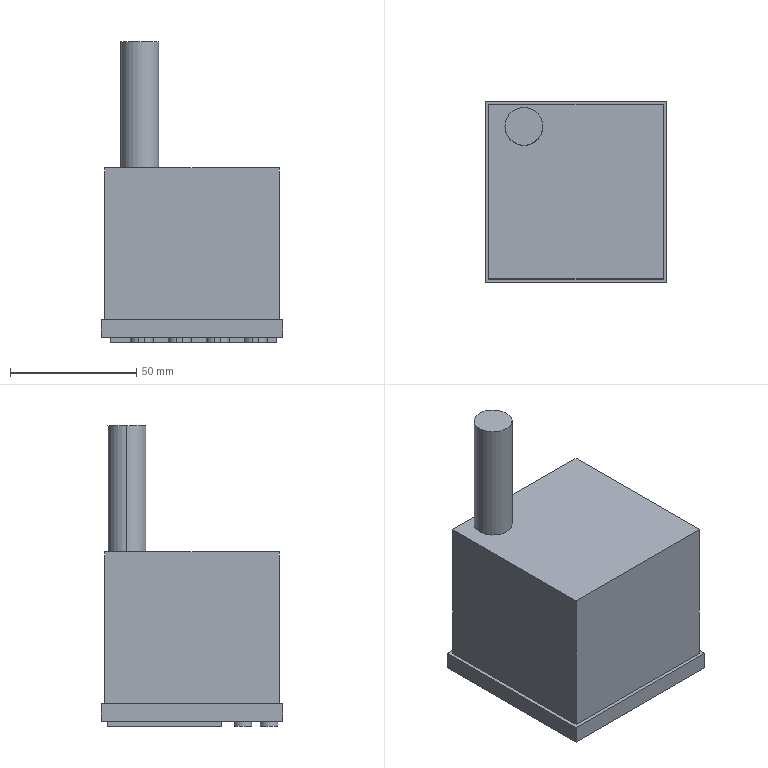Part | STEP file | Amplifier | 1 solid | 67 faces | box 72 x 72 x 119 mm | volume 337581 mm3 | plane 41 | cylinder 26 | commonest cylinder face diameters 6.961 x24 15 x2